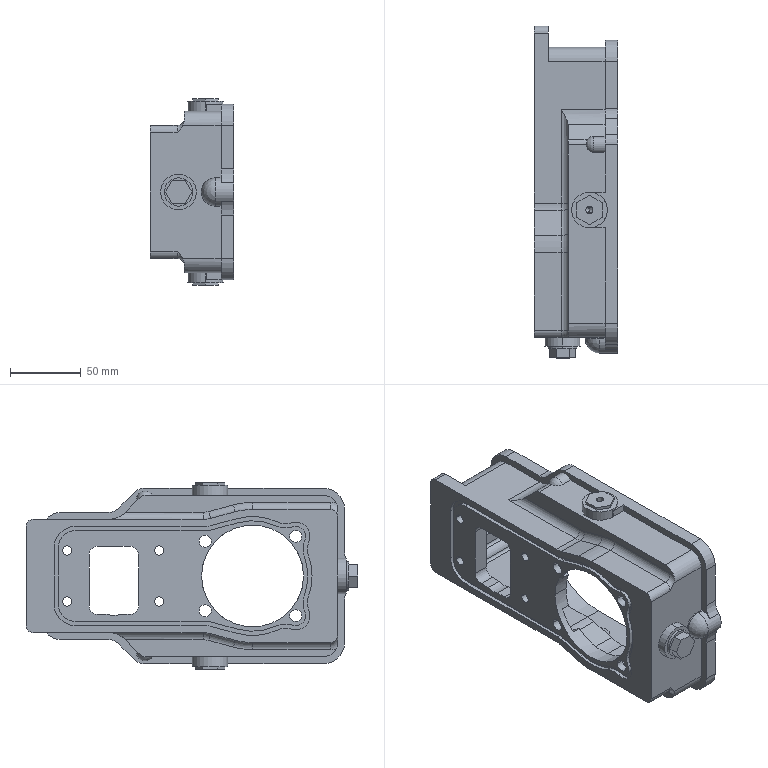Part | SolidWorks | features BaseBody 1 | 1 solid | 290 faces | box 59 x 234.4 x 132 mm | volume 372602 mm3 | cylinder 151 | plane 112 | cone 18 | torus 6 | sphere 3 | commonest cylinder face diameters 5 x18 20 x18 10 x14 8.5 x10 12 x10 30 x10